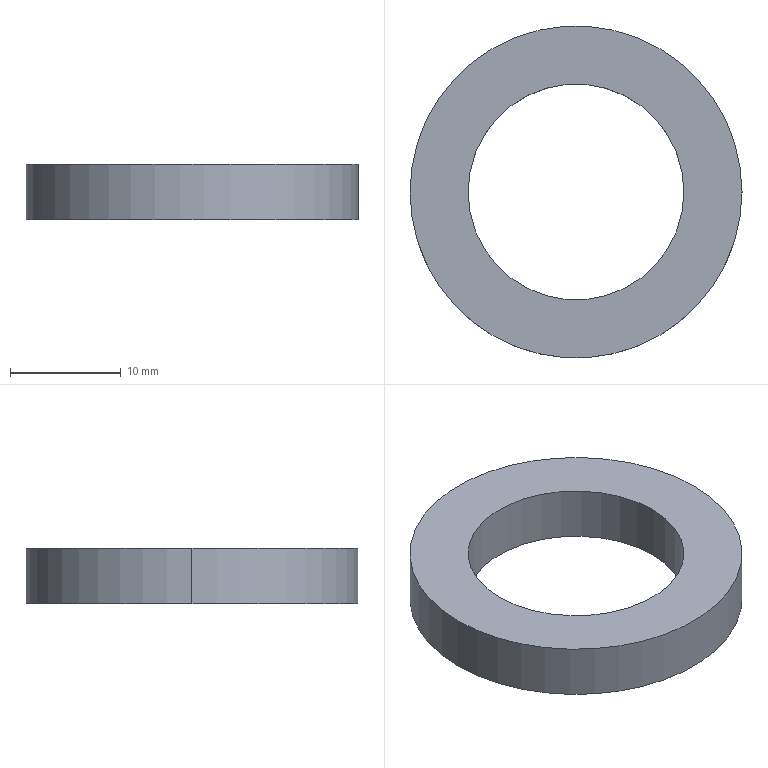Part | STEP file | 1 solid | 6 faces | box 30 x 30 x 5 mm | volume 2041 mm3 | cylinder 4 | plane 2 | commonest cylinder face diameters 19.5 x2 30 x2
STEP:
#1=CARTESIAN_POINT('',(0.,0.,0.));
#2=DIRECTION('',(0.,0.,1.));
#3=DIRECTION('',(1.,0.,0.));
#4=AXIS2_PLACEMENT_3D('',#1,#2,#3);
#5=CARTESIAN_POINT('',(-9.75,0.,5.));
#6=VERTEX_POINT('',#5);
#7=CARTESIAN_POINT('',(-9.75,0.,0.));
#8=VERTEX_POINT('',#7);
#9=CARTESIAN_POINT('',(-9.75,0.,5.));
#10=DIRECTION('',(0.,0.,-1.));
#11=VECTOR('',#10,1.);
#12=LINE('',#9,#11);
#13=CARTESIAN_POINT('',(0.,0.,5.));
#14=DIRECTION('',(0.,0.,-1.));
#15=DIRECTION('',(-1.,0.,0.));
#16=AXIS2_PLACEMENT_3D('',#13,#14,#15);
#17=CYLINDRICAL_SURFACE('',#16,9.75);
#18=CARTESIAN_POINT('',(6.283,0.));
#19=DIRECTION('',(0.,1.));
#20=VECTOR('',#19,1.);
#21=LINE('',#18,#20);
#22=(GEOMETRIC_REPRESENTATION_CONTEXT(2)PARAMETRIC_REPRESENTATION_CONTEXT()REPRESENTATION_CONTEXT('',''));
#23=DEFINITIONAL_REPRESENTATION('',(#21),#22);
#24=PCURVE('',#17,#23);
#25=CARTESIAN_POINT('',(0.,0.,5.));
#26=DIRECTION('',(0.,0.,-1.));
#27=DIRECTION('',(-1.,0.,0.));
#28=AXIS2_PLACEMENT_3D('',#25,#26,#27);
#29=CYLINDRICAL_SURFACE('',#28,9.75);
#30=CARTESIAN_POINT('',(0.,0.));
#31=DIRECTION('',(0.,1.));
#32=VECTOR('',#31,1.);
#33=LINE('',#30,#32);
#34=(GEOMETRIC_REPRESENTATION_CONTEXT(2)PARAMETRIC_REPRESENTATION_CONTEXT()REPRESENTATION_CONTEXT('',''));
#35=DEFINITIONAL_REPRESENTATION('',(#33),#34);
#36=PCURVE('',#29,#35);
#37=SURFACE_CURVE('',#12,(#24,#36),.PCURVE_S1.);
#38=EDGE_CURVE('',#6,#8,#37,.T.);
#39=ORIENTED_EDGE('',*,*,#38,.T.);
#40=CARTESIAN_POINT('',(9.75,0.,0.));
#41=VERTEX_POINT('',#40);
#42=CARTESIAN_POINT('',(0.,0.,0.));
#43=DIRECTION('',(0.,0.,1.));
#44=DIRECTION('',(1.,0.,0.));
#45=AXIS2_PLACEMENT_3D('',#42,#43,#44);
#46=CIRCLE('',#45,9.75);
#47=CARTESIAN_POINT('',(9.425,5.));
#48=DIRECTION('',(-1.,0.));
#49=VECTOR('',#48,1.);
#50=LINE('',#47,#49);
#51=(GEOMETRIC_REPRESENTATION_CONTEXT(2)PARAMETRIC_REPRESENTATION_CONTEXT()REPRESENTATION_CONTEXT('',''));
#52=DEFINITIONAL_REPRESENTATION('',(#50),#51);
#53=PCURVE('',#17,#52);
#54=CARTESIAN_POINT('',(0.,0.,0.));
#55=DIRECTION('',(0.,0.,1.));
#56=DIRECTION('',(1.,0.,0.));
#57=AXIS2_PLACEMENT_3D('',#54,#55,#56);
#58=PLANE('',#57);
#59=CARTESIAN_POINT('',(0.,0.));
#60=DIRECTION('',(1.,0.));
#61=AXIS2_PLACEMENT_2D('',#59,#60);
#62=CIRCLE('',#61,9.75);
#63=(GEOMETRIC_REPRESENTATION_CONTEXT(2)PARAMETRIC_REPRESENTATION_CONTEXT()REPRESENTATION_CONTEXT('',''));
#64=DEFINITIONAL_REPRESENTATION('',(#62),#63);
#65=PCURVE('',#58,#64);
#66=SURFACE_CURVE('',#46,(#53,#65),.PCURVE_S1.);
#67=EDGE_CURVE('',#8,#41,#66,.T.);
#68=ORIENTED_EDGE('',*,*,#67,.T.);
#69=CARTESIAN_POINT('',(9.75,0.,5.));
#70=VERTEX_POINT('',#69);
#71=CARTESIAN_POINT('',(9.75,0.,5.));
#72=DIRECTION('',(0.,0.,-1.));
#73=VECTOR('',#72,1.);
#74=LINE('',#71,#73);
#75=CARTESIAN_POINT('',(3.142,0.));
#76=DIRECTION('',(0.,1.));
#77=VECTOR('',#76,1.);
#78=LINE('',#75,#77);
#79=(GEOMETRIC_REPRESENTATION_CONTEXT(2)PARAMETRIC_REPRESENTATION_CONTEXT()REPRESENTATION_CONTEXT('',''));
#80=DEFINITIONAL_REPRESENTATION('',(#78),#79);
#81=PCURVE('',#17,#80);
#82=CARTESIAN_POINT('',(3.142,0.));
#83=DIRECTION('',(0.,1.));
#84=VECTOR('',#83,1.);
#85=LINE('',#82,#84);
#86=(GEOMETRIC_REPRESENTATION_CONTEXT(2)PARAMETRIC_REPRESENTATION_CONTEXT()REPRESENTATION_CONTEXT('',''));
#87=DEFINITIONAL_REPRESENTATION('',(#85),#86);
#88=PCURVE('',#29,#87);
#89=SURFACE_CURVE('',#74,(#81,#88),.PCURVE_S1.);
#90=EDGE_CURVE('',#70,#41,#89,.T.);
#91=ORIENTED_EDGE('',*,*,#90,.F.);
#92=CARTESIAN_POINT('',(0.,0.,5.));
#93=DIRECTION('',(0.,0.,1.));
#94=DIRECTION('',(1.,0.,0.));
#95=AXIS2_PLACEMENT_3D('',#92,#93,#94);
#96=CIRCLE('',#95,9.75);
#97=CARTESIAN_POINT('',(9.425,0.));
#98=DIRECTION('',(-1.,0.));
#99=VECTOR('',#98,1.);
#100=LINE('',#97,#99);
#101=(GEOMETRIC_REPRESENTATION_CONTEXT(2)PARAMETRIC_REPRESENTATION_CONTEXT()REPRESENTATION_CONTEXT('',''));
#102=DEFINITIONAL_REPRESENTATION('',(#100),#101);
#103=PCURVE('',#17,#102);
#104=CARTESIAN_POINT('',(0.,0.,5.));
#105=DIRECTION('',(0.,0.,1.));
#106=DIRECTION('',(1.,0.,0.));
#107=AXIS2_PLACEMENT_3D('',#104,#105,#106);
#108=PLANE('',#107);
#109=CARTESIAN_POINT('',(0.,0.));
#110=DIRECTION('',(1.,0.));
#111=AXIS2_PLACEMENT_2D('',#109,#110);
#112=CIRCLE('',#111,9.75);
#113=(GEOMETRIC_REPRESENTATION_CONTEXT(2)PARAMETRIC_REPRESENTATION_CONTEXT()REPRESENTATION_CONTEXT('',''));
#114=DEFINITIONAL_REPRESENTATION('',(#112),#113);
#115=PCURVE('',#108,#114);
#116=SURFACE_CURVE('',#96,(#103,#115),.PCURVE_S1.);
#117=EDGE_CURVE('',#6,#70,#116,.T.);
#118=ORIENTED_EDGE('',*,*,#117,.F.);
#119=EDGE_LOOP('',(#39,#68,#91,#118));
#120=FACE_BOUND('',#119,.F.);
#121=ADVANCED_FACE('',(#120),#17,.F.);
#122=CARTESIAN_POINT('',(15.,0.,5.));
#123=VERTEX_POINT('',#122);
#124=CARTESIAN_POINT('',(-15.,0.,5.));
#125=VERTEX_POINT('',#124);
#126=CARTESIAN_POINT('',(0.,0.,5.));
#127=DIRECTION('',(0.,0.,1.));
#128=DIRECTION('',(1.,0.,0.));
#129=AXIS2_PLACEMENT_3D('',#126,#127,#128);
#130=CIRCLE('',#129,15.);
#131=CARTESIAN_POINT('',(0.,0.,5.));
#132=DIRECTION('',(0.,0.,-1.));
#133=DIRECTION('',(-1.,0.,0.));
#134=AXIS2_PLACEMENT_3D('',#131,#132,#133);
#135=CYLINDRICAL_SURFACE('',#134,15.);
#136=CARTESIAN_POINT('',(3.142,0.));
#137=DIRECTION('',(-1.,0.));
#138=VECTOR('',#137,1.);
#139=LINE('',#136,#138);
#140=(GEOMETRIC_REPRESENTATION_CONTEXT(2)PARAMETRIC_REPRESENTATION_CONTEXT()REPRESENTATION_CONTEXT('',''));
#141=DEFINITIONAL_REPRESENTATION('',(#139),#140);
#142=PCURVE('',#135,#141);
#143=CARTESIAN_POINT('',(0.,0.));
#144=DIRECTION('',(1.,0.));
#145=AXIS2_PLACEMENT_2D('',#143,#144);
#146=CIRCLE('',#145,15.);
#147=(GEOMETRIC_REPRESENTATION_CONTEXT(2)PARAMETRIC_REPRESENTATION_CONTEXT()REPRESENTATION_CONTEXT('',''));
#148=DEFINITIONAL_REPRESENTATION('',(#146),#147);
#149=PCURVE('',#108,#148);
#150=SURFACE_CURVE('',#130,(#142,#149),.PCURVE_S1.);
#151=EDGE_CURVE('',#123,#125,#150,.T.);
#152=ORIENTED_EDGE('',*,*,#151,.F.);
#153=CARTESIAN_POINT('',(15.,0.,0.));
#154=VERTEX_POINT('',#153);
#155=CARTESIAN_POINT('',(15.,0.,5.));
#156=DIRECTION('',(0.,0.,-1.));
#157=VECTOR('',#156,1.);
#158=LINE('',#155,#157);
#159=CARTESIAN_POINT('',(3.142,0.));
#160=DIRECTION('',(0.,1.));
#161=VECTOR('',#160,1.);
#162=LINE('',#159,#161);
#163=(GEOMETRIC_REPRESENTATION_CONTEXT(2)PARAMETRIC_REPRESENTATION_CONTEXT()REPRESENTATION_CONTEXT('',''));
#164=DEFINITIONAL_REPRESENTATION('',(#162),#163);
#165=PCURVE('',#135,#164);
#166=CARTESIAN_POINT('',(0.,0.,5.));
#167=DIRECTION('',(0.,0.,-1.));
#168=DIRECTION('',(-1.,0.,0.));
#169=AXIS2_PLACEMENT_3D('',#166,#167,#168);
#170=CYLINDRICAL_SURFACE('',#169,15.);
#171=CARTESIAN_POINT('',(3.142,0.));
#172=DIRECTION('',(0.,1.));
#173=VECTOR('',#172,1.);
#174=LINE('',#171,#173);
#175=(GEOMETRIC_REPRESENTATION_CONTEXT(2)PARAMETRIC_REPRESENTATION_CONTEXT()REPRESENTATION_CONTEXT('',''));
#176=DEFINITIONAL_REPRESENTATION('',(#174),#175);
#177=PCURVE('',#170,#176);
#178=SURFACE_CURVE('',#158,(#165,#177),.PCURVE_S1.);
#179=EDGE_CURVE('',#123,#154,#178,.T.);
#180=ORIENTED_EDGE('',*,*,#179,.T.);
#181=CARTESIAN_POINT('',(-15.,0.,0.));
#182=VERTEX_POINT('',#181);
#183=CARTESIAN_POINT('',(0.,0.,0.));
#184=DIRECTION('',(0.,0.,1.));
#185=DIRECTION('',(1.,0.,0.));
#186=AXIS2_PLACEMENT_3D('',#183,#184,#185);
#187=CIRCLE('',#186,15.);
#188=CARTESIAN_POINT('',(3.142,5.));
#189=DIRECTION('',(-1.,0.));
#190=VECTOR('',#189,1.);
#191=LINE('',#188,#190);
#192=(GEOMETRIC_REPRESENTATION_CONTEXT(2)PARAMETRIC_REPRESENTATION_CONTEXT()REPRESENTATION_CONTEXT('',''));
#193=DEFINITIONAL_REPRESENTATION('',(#191),#192);
#194=PCURVE('',#135,#193);
#195=CARTESIAN_POINT('',(0.,0.));
#196=DIRECTION('',(1.,0.));
#197=AXIS2_PLACEMENT_2D('',#195,#196);
#198=CIRCLE('',#197,15.);
#199=(GEOMETRIC_REPRESENTATION_CONTEXT(2)PARAMETRIC_REPRESENTATION_CONTEXT()REPRESENTATION_CONTEXT('',''));
#200=DEFINITIONAL_REPRESENTATION('',(#198),#199);
#201=PCURVE('',#58,#200);
#202=SURFACE_CURVE('',#187,(#194,#201),.PCURVE_S1.);
#203=EDGE_CURVE('',#154,#182,#202,.T.);
#204=ORIENTED_EDGE('',*,*,#203,.T.);
#205=CARTESIAN_POINT('',(-15.,0.,5.));
#206=DIRECTION('',(0.,0.,-1.));
#207=VECTOR('',#206,1.);
#208=LINE('',#205,#207);
#209=CARTESIAN_POINT('',(0.,0.));
#210=DIRECTION('',(0.,1.));
#211=VECTOR('',#210,1.);
#212=LINE('',#209,#211);
#213=(GEOMETRIC_REPRESENTATION_CONTEXT(2)PARAMETRIC_REPRESENTATION_CONTEXT()REPRESENTATION_CONTEXT('',''));
#214=DEFINITIONAL_REPRESENTATION('',(#212),#213);
#215=PCURVE('',#135,#214);
#216=CARTESIAN_POINT('',(6.283,0.));
#217=DIRECTION('',(0.,1.));
#218=VECTOR('',#217,1.);
#219=LINE('',#216,#218);
#220=(GEOMETRIC_REPRESENTATION_CONTEXT(2)PARAMETRIC_REPRESENTATION_CONTEXT()REPRESENTATION_CONTEXT('',''));
#221=DEFINITIONAL_REPRESENTATION('',(#219),#220);
#222=PCURVE('',#170,#221);
#223=SURFACE_CURVE('',#208,(#215,#222),.PCURVE_S1.);
#224=EDGE_CURVE('',#125,#182,#223,.T.);
#225=ORIENTED_EDGE('',*,*,#224,.F.);
#226=EDGE_LOOP('',(#152,#180,#204,#225));
#227=FACE_BOUND('',#226,.T.);
#228=ADVANCED_FACE('',(#227),#135,.T.);
#229=CARTESIAN_POINT('',(0.,0.,5.));
#230=DIRECTION('',(0.,0.,1.));
#231=DIRECTION('',(1.,0.,0.));
#232=AXIS2_PLACEMENT_3D('',#229,#230,#231);
#233=CIRCLE('',#232,15.);
#234=CARTESIAN_POINT('',(0.,0.));
#235=DIRECTION('',(1.,0.));
#236=AXIS2_PLACEMENT_2D('',#234,#235);
#237=CIRCLE('',#236,15.);
#238=(GEOMETRIC_REPRESENTATION_CONTEXT(2)PARAMETRIC_REPRESENTATION_CONTEXT()REPRESENTATION_CONTEXT('',''));
#239=DEFINITIONAL_REPRESENTATION('',(#237),#238);
#240=PCURVE('',#108,#239);
#241=CARTESIAN_POINT('',(9.425,0.));
#242=DIRECTION('',(-1.,0.));
#243=VECTOR('',#242,1.);
#244=LINE('',#241,#243);
#245=(GEOMETRIC_REPRESENTATION_CONTEXT(2)PARAMETRIC_REPRESENTATION_CONTEXT()REPRESENTATION_CONTEXT('',''));
#246=DEFINITIONAL_REPRESENTATION('',(#244),#245);
#247=PCURVE('',#170,#246);
#248=SURFACE_CURVE('',#233,(#240,#247),.PCURVE_S1.);
#249=EDGE_CURVE('',#125,#123,#248,.T.);
#250=ORIENTED_EDGE('',*,*,#249,.T.);
#251=ORIENTED_EDGE('',*,*,#151,.T.);
#252=EDGE_LOOP('',(#250,#251));
#253=FACE_BOUND('',#252,.T.);
#254=ORIENTED_EDGE('',*,*,#117,.F.);
#255=CARTESIAN_POINT('',(0.,0.,5.));
#256=DIRECTION('',(0.,0.,1.));
#257=DIRECTION('',(1.,0.,0.));
#258=AXIS2_PLACEMENT_3D('',#255,#256,#257);
#259=CIRCLE('',#258,9.75);
#260=CARTESIAN_POINT('',(0.,0.));
#261=DIRECTION('',(1.,0.));
#262=AXIS2_PLACEMENT_2D('',#260,#261);
#263=CIRCLE('',#262,9.75);
#264=(GEOMETRIC_REPRESENTATION_CONTEXT(2)PARAMETRIC_REPRESENTATION_CONTEXT()REPRESENTATION_CONTEXT('',''));
#265=DEFINITIONAL_REPRESENTATION('',(#263),#264);
#266=PCURVE('',#108,#265);
#267=CARTESIAN_POINT('',(3.142,0.));
#268=DIRECTION('',(-1.,0.));
#269=VECTOR('',#268,1.);
#270=LINE('',#267,#269);
#271=(GEOMETRIC_REPRESENTATION_CONTEXT(2)PARAMETRIC_REPRESENTATION_CONTEXT()REPRESENTATION_CONTEXT('',''));
#272=DEFINITIONAL_REPRESENTATION('',(#270),#271);
#273=PCURVE('',#29,#272);
#274=SURFACE_CURVE('',#259,(#266,#273),.PCURVE_S1.);
#275=EDGE_CURVE('',#70,#6,#274,.T.);
#276=ORIENTED_EDGE('',*,*,#275,.F.);
#277=EDGE_LOOP('',(#254,#276));
#278=FACE_BOUND('',#277,.T.);
#279=ADVANCED_FACE('',(#253,#278),#108,.T.);
#280=CARTESIAN_POINT('',(0.,0.,0.));
#281=DIRECTION('',(0.,0.,1.));
#282=DIRECTION('',(1.,0.,0.));
#283=AXIS2_PLACEMENT_3D('',#280,#281,#282);
#284=CIRCLE('',#283,15.);
#285=CARTESIAN_POINT('',(0.,0.));
#286=DIRECTION('',(1.,0.));
#287=AXIS2_PLACEMENT_2D('',#285,#286);
#288=CIRCLE('',#287,15.);
#289=(GEOMETRIC_REPRESENTATION_CONTEXT(2)PARAMETRIC_REPRESENTATION_CONTEXT()REPRESENTATION_CONTEXT('',''));
#290=DEFINITIONAL_REPRESENTATION('',(#288),#289);
#291=PCURVE('',#58,#290);
#292=CARTESIAN_POINT('',(9.425,5.));
#293=DIRECTION('',(-1.,0.));
#294=VECTOR('',#293,1.);
#295=LINE('',#292,#294);
#296=(GEOMETRIC_REPRESENTATION_CONTEXT(2)PARAMETRIC_REPRESENTATION_CONTEXT()REPRESENTATION_CONTEXT('',''));
#297=DEFINITIONAL_REPRESENTATION('',(#295),#296);
#298=PCURVE('',#170,#297);
#299=SURFACE_CURVE('',#284,(#291,#298),.PCURVE_S1.);
#300=EDGE_CURVE('',#182,#154,#299,.T.);
#301=ORIENTED_EDGE('',*,*,#300,.F.);
#302=ORIENTED_EDGE('',*,*,#203,.F.);
#303=EDGE_LOOP('',(#301,#302));
#304=FACE_BOUND('',#303,.T.);
#305=ORIENTED_EDGE('',*,*,#67,.T.);
#306=CARTESIAN_POINT('',(0.,0.,0.));
#307=DIRECTION('',(0.,0.,1.));
#308=DIRECTION('',(1.,0.,0.));
#309=AXIS2_PLACEMENT_3D('',#306,#307,#308);
#310=CIRCLE('',#309,9.75);
#311=CARTESIAN_POINT('',(0.,0.));
#312=DIRECTION('',(1.,0.));
#313=AXIS2_PLACEMENT_2D('',#311,#312);
#314=CIRCLE('',#313,9.75);
#315=(GEOMETRIC_REPRESENTATION_CONTEXT(2)PARAMETRIC_REPRESENTATION_CONTEXT()REPRESENTATION_CONTEXT('',''));
#316=DEFINITIONAL_REPRESENTATION('',(#314),#315);
#317=PCURVE('',#58,#316);
#318=CARTESIAN_POINT('',(3.142,5.));
#319=DIRECTION('',(-1.,0.));
#320=VECTOR('',#319,1.);
#321=LINE('',#318,#320);
#322=(GEOMETRIC_REPRESENTATION_CONTEXT(2)PARAMETRIC_REPRESENTATION_CONTEXT()REPRESENTATION_CONTEXT('',''));
#323=DEFINITIONAL_REPRESENTATION('',(#321),#322);
#324=PCURVE('',#29,#323);
#325=SURFACE_CURVE('',#310,(#317,#324),.PCURVE_S1.);
#326=EDGE_CURVE('',#41,#8,#325,.T.);
#327=ORIENTED_EDGE('',*,*,#326,.T.);
#328=EDGE_LOOP('',(#305,#327));
#329=FACE_BOUND('',#328,.T.);
#330=ADVANCED_FACE('',(#304,#329),#58,.F.);
#331=ORIENTED_EDGE('',*,*,#179,.F.);
#332=ORIENTED_EDGE('',*,*,#249,.F.);
#333=ORIENTED_EDGE('',*,*,#224,.T.);
#334=ORIENTED_EDGE('',*,*,#300,.T.);
#335=EDGE_LOOP('',(#331,#332,#333,#334));
#336=FACE_BOUND('',#335,.T.);
#337=ADVANCED_FACE('',(#336),#170,.T.);
#338=ORIENTED_EDGE('',*,*,#326,.T.);
#339=ORIENTED_EDGE('',*,*,#38,.F.);
#340=ORIENTED_EDGE('',*,*,#275,.F.);
#341=ORIENTED_EDGE('',*,*,#90,.T.);
#342=EDGE_LOOP('',(#338,#339,#340,#341));
#343=FACE_BOUND('',#342,.F.);
#344=ADVANCED_FACE('',(#343),#29,.F.);
#345=CLOSED_SHELL('',(#121,#228,#279,#330,#337,#344));
#346=MANIFOLD_SOLID_BREP('',#345);
#347=(LENGTH_UNIT()NAMED_UNIT(*)SI_UNIT(.MILLI.,.METRE.));
#348=UNCERTAINTY_MEASURE_WITH_UNIT(LENGTH_MEASURE(0.0000001),#347,'','');
#349=(NAMED_UNIT(*)PLANE_ANGLE_UNIT()SI_UNIT($,.RADIAN.));
#350=(NAMED_UNIT(*)SI_UNIT($,.STERADIAN.)SOLID_ANGLE_UNIT());
#351=(GEOMETRIC_REPRESENTATION_CONTEXT(3)GLOBAL_UNCERTAINTY_ASSIGNED_CONTEXT((#348))GLOBAL_UNIT_ASSIGNED_CONTEXT((#347,#349,#350))REPRESENTATION_CONTEXT('',''));
#352=ADVANCED_BREP_SHAPE_REPRESENTATION('',(#4,#346),#351);